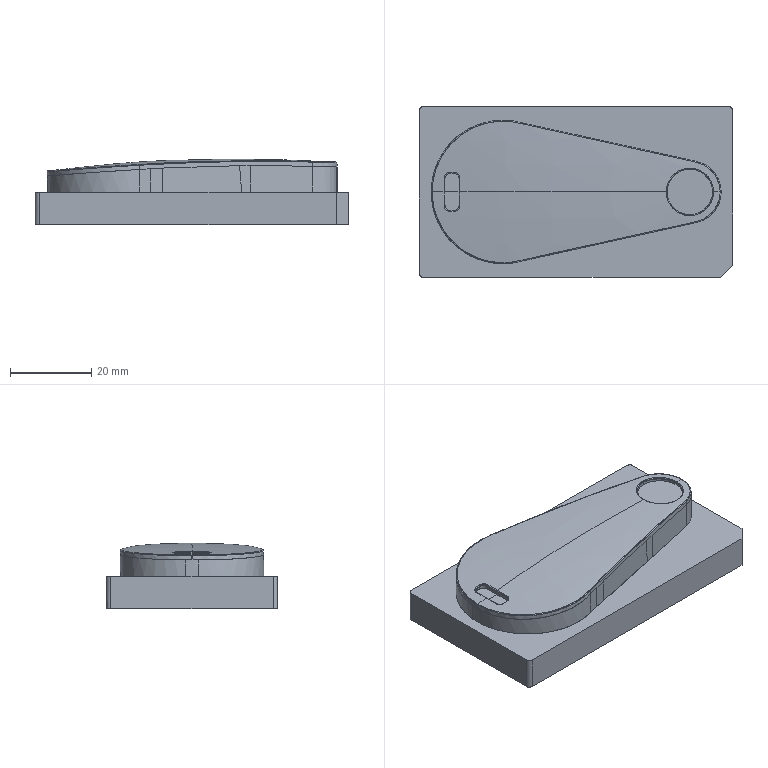NC program | PowerMill | posted with a generic post | part box 77 x 42 x 16.114 mm
Lines 5463 to 6450 of 230441:
N5560 M6
N5561 S18000 M03
N5562 G00 G90 X0.0 Y0.0
N5563 G43 Z9.8037 H2
N5564
N5565 G05 P10000 R4
N5566 X25.6106 Y4.3467
N5567 Z0.8002
N5568 G01 Z-0.3998 F3600.0
N5569 X25.5892 Y4.3418 F6000.0
N5570 G03 X25.4406 Y4.1045 I0.0443 J-0.193
N5571 G01 X25.4866 Y3.9044
N5572 X25.4887 Y3.4164
N5573 X25.3787 Y2.998
N5574 X25.0805 Y2.4403
N5575 X24.5954 Y1.4642
N5576 X24.4343 Y0.9761
N5577 X24.3483 Y0.4881
N5578 X24.3167 Y0.0
N5579 X24.3478 Y-0.4881
N5580 X24.4026 Y-0.8353
N5581 X24.5953 Y-1.4642
N5582 X24.8242 Y-1.9522
N5583 X25.3481 Y-2.9283
N5584 X25.4887 Y-3.4164
N5585 X25.4785 Y-3.9044
N5586 X25.4342 Y-4.1119
N5587 G00 Z3.6074
N5588 G01 X27.1301 Y-2.5287 F10000.0
N5589 G00 Z0.6074
N5590 G01 Z-0.5926 F3600.0
N5591 X27.116 Y-2.5456 F6000.0
N5592 G03 X27.1414 Y-2.8245 I0.1521 J-0.1268
N5593 G01 X28.3826 Y-3.8587
N5594 X28.5768 Y-3.9044
N5595 X28.7951 Y-4.0192
N5596 X29.3579 Y-4.3925
N5597 X29.7167 Y-4.8805
N5598 X29.9105 Y-5.3686
N5599 X29.9759 Y-5.8566
N5600 X29.7712 Y-6.6239
N5601 X29.2812 Y-7.3208
N5602 X28.8585 Y-7.8088
N5603 X28.8118 Y-7.8327
N5604 X28.7708 Y-7.8653
N5605 X28.3555 Y-8.2969
N5606 X27.3258 Y-9.273
N5607 X26.8429 Y-9.654
N5608 X26.3548 Y-9.9782
N5609 X25.8668 Y-10.1481
N5610 X23.9146 Y-10.6849
N5611 X19.5221 Y-11.695
N5612 X12.2013 Y-13.2735
N5613 X9.9964 Y-13.6655
N5614 X9.7611 Y-13.6988
N5615 X9.273 Y-13.7039
N5616 X7.8088 Y-13.6203
N5617 X6.8327 Y-13.5369
N5618 X2.4403 Y-12.8888
N5619 X1.4642 Y-12.6222
N5620 X0.225 Y-12.2013
N5621 X-2.4782 Y-11.2252
N5622 X-4.1922 Y-10.2491
N5623 X-6.6783 Y-8.2969
N5624 X-7.2227 Y-7.8088
N5625 X-7.5763 Y-7.3208
N5626 X-8.8466 Y-5.3686
N5627 X-9.0736 Y-4.8805
N5628 X-9.2569 Y-4.3925
N5629 X-9.273 Y-4.2801
N5630 X-9.4151 Y-3.9044
N5631 X-9.7611 Y-2.7958
N5632 X-9.8455 Y-2.4403
N5633 X-10.12 Y0.0
N5634 X-10.0611 Y0.4881
N5635 X-9.5893 Y3.4164
N5636 X-9.4579 Y3.9044
N5637 X-9.2392 Y4.3925
N5638 X-8.4707 Y5.8566
N5639 X-8.2969 Y6.2312
N5640 X-7.7643 Y7.0243
N5641 X-7.2192 Y7.8088
N5642 X-6.8327 Y8.1753
N5643 X-6.3447 Y8.5793
N5644 X-4.2536 Y10.2491
N5645 X-2.9283 Y11.0116
N5646 X-2.4011 Y11.2252
N5647 X0.9761 Y12.5318
N5648 X1.6269 Y12.6894
N5649 X5.3686 Y13.3735
N5650 X7.8088 Y13.6136
N5651 X9.273 Y13.7182
N5652 X9.7611 Y13.7068
N5653 X12.2013 Y13.2736
N5654 X19.4399 Y11.7133
N5655 X24.4026 Y10.5617
N5656 X25.8668 Y10.1488
N5657 X26.3548 Y9.9675
N5658 X26.6924 Y9.7611
N5659 X27.8709 Y8.7849
N5660 X28.3071 Y8.3429
N5661 X28.3784 Y8.2969
N5662 X28.7951 Y7.8593
N5663 X29.2752 Y7.3208
N5664 X29.7712 Y6.6241
N5665 X29.9436 Y5.8566
N5666 X29.9106 Y5.3686
N5667 X29.7167 Y4.8805
N5668 X29.3579 Y4.3925
N5669 X28.7951 Y4.0127
N5670 X28.5768 Y3.9044
N5671 X27.819 Y3.7276
N5672 X27.331 Y3.636
N5673 X26.8429 Y3.4818
N5674 X26.3548 Y3.2494
N5675 X25.8668 Y2.9362
N5676 X25.3787 Y2.5085
N5677 X24.95 Y1.9522
N5678 X24.6865 Y1.4642
N5679 X24.5104 Y0.9761
N5680 X24.4102 Y0.4881
N5681 X24.3727 Y0.0
N5682 X24.4026 Y-0.4368
N5683 X24.5106 Y-0.9761
N5684 X24.6871 Y-1.4642
N5685 X24.95 Y-1.9522
N5686 X25.3787 Y-2.5062
N5687 X25.8513 Y-2.9283
N5688 X26.3548 Y-3.2502
N5689 X26.6937 Y-3.4164
N5690 X27.331 Y-3.6387
N5691 X27.3463 Y-3.6415
N5692 X27.819 Y-3.7262
N5693 X28.3826 Y-3.8587
N5694 G00 Z3.4146
N5695 G01 X35.8789 Y-0.8619 F10000.0
N5696 G00 Z0.4146
N5697 G01 Z-0.7854 F3600.0
N5698 X35.6662 Y-0.9181 F6000.0
N5699 X35.1553 Y-1.0529
N5700 X35.2638 Y-1.4642
N5701 X35.3532 Y-1.9522
N5702 X35.3635 Y-2.4403
N5703 X35.2988 Y-2.9283
N5704 X35.0735 Y-3.9044
N5705 X34.6517 Y-5.2467
N5706 X33.9876 Y-6.8327
N5707 X33.6756 Y-7.3561
N5708 X33.3034 Y-7.8088
N5709 X32.6995 Y-8.2555
N5710 X32.2115 Y-8.5608
N5711 X31.7554 Y-8.7849
N5712 X30.7473 Y-9.1776
N5713 X29.7712 Y-9.4515
N5714 X26.3135 Y-10.2491
N5715 X16.5938 Y-12.3992
N5716 X5.8566 Y-14.7403
N5717 X4.3934 Y-15.0298
N5718 X2.9283 Y-15.3093
N5719 X1.9522 Y-15.4353
N5720 X1.4642 Y-15.451
N5721 X0.4881 Y-15.2623
N5722 X-1.9522 Y-14.6462
N5723 X-2.4403 Y-14.4911
N5724 X-3.246 Y-14.1535
N5725 X-3.4164 Y-14.0596
N5726 X-4.3925 Y-13.6327
N5727 X-5.4918 Y-13.1774
N5728 X-6.3447 Y-12.7858
N5729 X-6.8327 Y-12.5383
N5730 X-7.8088 Y-11.7777
N5731 X-9.5744 Y-10.2491
N5732 X-10.0631 Y-9.7611
N5733 X-10.7372 Y-8.9567
N5734 X-11.7133 Y-7.574
N5735 X-11.8564 Y-7.3208
N5736 X-12.2728 Y-6.3447
N5737 X-12.8568 Y-4.8805
N5738 X-13.4383 Y-2.4403
N5739 X-13.5139 Y-1.4642
N5740 X-13.6555 Y0.0
N5741 X-13.2625 Y3.4164
N5742 X-13.1774 Y3.8738
N5743 X-13.0029 Y4.3925
N5744 X-12.1989 Y6.3447
N5745 X-11.8442 Y7.3208
N5746 X-11.7133 Y7.556
N5747 X-10.8773 Y8.7849
N5748 X-10.0633 Y9.7611
N5749 X-9.7611 Y10.0829
N5750 X-8.7849 Y11.0004
N5751 X-7.3131 Y12.2013
N5752 X-6.8327 Y12.5382
N5753 X-6.3447 Y12.7951
N5754 X-4.482 Y13.6655
N5755 X-2.9283 Y14.323
N5756 X-0.9761 Y14.8925
N5757 X0.4881 Y15.2705
N5758 X1.4642 Y15.4511
N5759 X1.9522 Y15.4349
N5760 X2.9283 Y15.3086
N5761 X5.8566 Y14.7382
N5762 X7.8088 Y14.3235
N5763 X23.9146 Y10.7827
N5764 X29.7712 Y9.4523
N5765 X30.7473 Y9.1777
N5766 X31.7234 Y8.7999
N5767 X32.2115 Y8.5582
N5768 X32.6995 Y8.2553
N5769 X33.3046 Y7.8088
N5770 X33.6756 Y7.3973
N5771 X33.9847 Y6.8327
N5772 X34.4222 Y5.8566
N5773 X34.6155 Y5.3686
N5774 X34.9322 Y4.3925
N5775 X35.2987 Y2.9283
N5776 X35.3635 Y2.4403
N5777 X35.3532 Y1.9522
N5778 X35.2638 Y1.4642
N5779 X35.1398 Y1.0387
N5780 X35.0622 Y0.9761
N5781 X34.6517 Y0.427
N5782 X34.1637 Y0.1714
N5783 X33.6756 Y0.0491
N5784 X33.1876 Y0.0475
N5785 X32.6995 Y0.1706
N5786 X32.2529 Y0.4881
N5787 X31.7234 Y0.9959
N5788 X31.482 Y1.4642
N5789 X31.2354 Y1.8465
N5790 X30.7585 Y2.4403
N5791 X30.2593 Y2.8756
N5792 X29.7712 Y3.1695
N5793 X29.2832 Y3.3861
N5794 X28.7951 Y3.528
N5795 X28.4637 Y3.5738
N5796 X28.2514 Y1.7284
N5797 G02 X29.5105 Y0.833 I-0.183 J-1.5903
N5798 G01 X29.7351 Y0.367
N5799 G02 X29.7651 Y-0.2566 I-0.7207 J-0.3473
N5800 G01 X29.617 Y-0.6592
N5801 G02 X26.5398 Y-0.3983 I-1.5028 J0.5532
N5802 G01 X26.4945 Y-0.1541
N5803 G02 X28.2514 Y1.7284 I1.5739 J0.2922
N5804 G01 X28.4637 Y3.5738
N5805 X28.3071 Y3.5954
N5806 X27.819 Y3.5943
N5807 X27.331 Y3.5453
N5808 X26.8429 Y3.421
N5809 X26.3548 Y3.2163
N5810 X25.8819 Y2.9283
N5811 X25.3787 Y2.4945
N5812 X24.95 Y1.9522
N5813 X24.6868 Y1.4642
N5814 X24.5104 Y0.9761
N5815 X24.4102 Y0.4881
N5816 X24.3727 Y0.0
N5817 X24.4026 Y-0.4366
N5818 X24.5143 Y-0.9761
N5819 X24.6822 Y-1.4503
N5820 X24.6878 Y-1.4644
N5821 X24.6945 Y-1.478
N5822 X24.9109 Y-1.8796
N5823 X25.3787 Y-2.4942
N5824 X25.8668 Y-2.9171
N5825 X26.3548 Y-3.2156
N5826 X26.838 Y-3.4164
N5827 X27.331 Y-3.5441
N5828 X27.819 Y-3.5974
N5829 X28.3071 Y-3.5959
N5830 X28.7951 Y-3.528
N5831 X29.2013 Y-3.4164
N5832 X29.7712 Y-3.1695
N5833 X30.1837 Y-2.9283
N5834 X30.513 Y-2.6751
N5835 X30.7473 Y-2.451
N5836 X31.1615 Y-1.9522
N5837 X31.482 Y-1.4642
N5838 X31.7295 Y-0.9761
N5839 X32.2115 Y-0.4065
N5840 X32.6995 Y-0.1452
N5841 X33.1876 Y-0.0416
N5842 X33.6756 Y-0.044
N5843 X34.1637 Y-0.1484
N5844 X34.6817 Y-0.4881
N5845 X35.0187 Y-0.9203
N5846 X35.0641 Y-0.9629
N5847 X35.1208 Y-0.9884
N5848 X35.1302 Y-0.9915
N5849 X35.1398 Y-0.9941
N5850 X35.1553 Y-1.0529
N5851 X35.6662 Y-0.9181
N5852 X38.5413 Y0.1203 Z-0.9782
N5853 X38.5227 Y0.1321
N5854 G03 X38.2495 Y0.0705 I-0.1058 J-0.1674
N5855 G01 X37.508 Y-1.1028
N5856 X37.4718 Y-1.4642
N5857 X37.2745 Y-2.4403
N5858 X36.9717 Y-3.4164
N5859 X36.604 Y-4.2751
N5860 X36.1159 Y-5.1424
N5861 X35.6243 Y-5.8566
N5862 X35.2324 Y-6.3447
N5863 X34.7776 Y-6.8327
N5864 X34.2506 Y-7.3208
N5865 X33.6405 Y-7.8088
N5866 X32.9051 Y-8.2969
N5867 X31.9708 Y-8.7849
N5868 X31.2354 Y-9.0837
N5869 X30.2593 Y-9.3761
N5870 X26.4891 Y-10.2085
N5871 X26.4882 Y-10.2088
N5872 X26.3135 Y-10.2491
N5873 X16.5938 Y-12.3992
N5874 X14.5691 Y-12.8406
N5875 X1.9925 Y-15.6177
N5876 X-0.4881 Y-16.1386
N5877 X-2.4403 Y-16.5026
N5878 X-3.2654 Y-16.5938
N5879 X-3.9044 Y-16.5999
N5880 X-4.3925 Y-16.4683
N5881 X-6.3447 Y-15.7841
N5882 X-6.7264 Y-15.6177
N5883 X-8.7849 Y-14.5464
N5884 X-10.7372 Y-13.2261
N5885 X-11.7133 Y-12.294
N5886 X-11.837 Y-12.2013
N5887 X-12.2013 Y-11.7945
N5888 X-13.6655 Y-9.9471
N5889 X-14.1139 Y-9.273
N5890 X-14.6628 Y-8.2969
N5891 X-15.1116 Y-7.3208
N5892 X-15.5806 Y-5.8566
N5893 X-15.8781 Y-4.8805
N5894 X-15.9874 Y-4.3925
N5895 X-16.3348 Y-2.4403
N5896 X-16.4619 Y-0.4881
N5897 X-16.5158 Y0.0
N5898 X-16.2262 Y3.4164
N5899 X-15.9983 Y4.3925
N5900 X-15.4109 Y6.3447
N5901 X-15.296 Y6.8327
N5902 X-15.1247 Y7.3208
N5903 X-14.4132 Y8.7849
N5904 X-14.1374 Y9.273
N5905 X-13.8175 Y9.7611
N5906 X-13.0974 Y10.7372
N5907 X-12.285 Y11.7133
N5908 X-11.8245 Y12.208
N5909 X-11.3501 Y12.6894
N5910 X-10.7372 Y13.2181
N5911 X-9.4035 Y14.1535
N5912 X-8.7849 Y14.5248
N5913 X-6.8327 Y15.5703
N5914 X-6.3447 Y15.7858
N5915 X-4.3925 Y16.4679
N5916 X-3.9044 Y16.5929
N5917 X-3.4164 Y16.6082
N5918 X-2.4403 Y16.5026
N5919 X-0.4881 Y16.1392
N5920 X1.4642 Y15.7293
N5921 X29.2832 Y9.6002
N5922 X30.6571 Y9.273
N5923 X31.2354 Y9.0811
N5924 X31.9708 Y8.7849
N5925 X32.9053 Y8.2969
N5926 X33.6756 Y7.7844
N5927 X34.2507 Y7.3208
N5928 X34.6517 Y6.9583
N5929 X35.1398 Y6.4481
N5930 X35.6278 Y5.8512
N5931 X35.9751 Y5.3686
N5932 X36.5433 Y4.3925
N5933 X36.7728 Y3.9044
N5934 X37.092 Y3.0703
N5935 X37.2745 Y2.4403
N5936 X37.4718 Y1.4642
N5937 X37.5697 Y0.4881
N5938 Y-0.4881
N5939 X37.508 Y-1.1028
N5940 X38.6013 Y0.1297 Z-1.171
N5941 X38.5827 Y0.1415
N5942 G03 X38.3094 Y0.0807 I-0.1063 J-0.1671
N5943 G01 X37.5534 Y-1.1075
N5944 X37.5165 Y-1.4642
N5945 X37.3193 Y-2.4403
N5946 X37.092 Y-3.1878
N5947 X36.8083 Y-3.9044
N5948 X36.604 Y-4.3287
N5949 X36.1159 Y-5.1943
N5950 X35.6525 Y-5.8566
N5951 X35.2503 Y-6.3447
N5952 X34.796 Y-6.8327
N5953 X34.274 Y-7.3208
N5954 X33.6756 Y-7.7972
N5955 X33.1876 Y-8.1303
N5956 X32.9821 Y-8.2457
N5957 X32.9051 Y-8.2969
N5958 X32.7049 Y-8.4014
N5959 X32.2115 Y-8.6785
N5960 X31.7234 Y-8.9028
N5961 X31.3486 Y-9.0377
N5962 X31.25 Y-9.0785
N5963 X31.1479 Y-9.1099
N5964 X30.7473 Y-9.254
N5965 X30.2593 Y-9.3836
N5966 X2.0338 Y-15.6177
N5967 X-4.7201 Y-17.0818
N5968 X-6.8327 Y-17.4646
N5969 X-7.8088 Y-17.5274
N5970 X-8.2969 Y-17.4459
N5971 X-9.273 Y-17.0261
N5972 X-10.178 Y-16.5938
N5973 X-11.2252 Y-15.9695
N5974 X-13.0937 Y-14.6416
N5975 X-13.6831 Y-14.1535
N5976 X-14.1434 Y-13.6655
N5977 X-14.6416 Y-13.085
N5978 X-15.6177 Y-11.8131
N5979 X-15.9656 Y-11.2252
N5980 X-17.0688 Y-9.273
N5981 X-17.87 Y-7.3208
N5982 X-18.0273 Y-6.8327
N5983 X-18.0579 Y-6.6332
N5984 X-18.3548 Y-5.3686
N5985 X-18.5641 Y-4.3925
N5986 X-18.8405 Y-2.4403
N5987 X-18.9401 Y-0.4881
N5988 X-18.9947 Y0.0
N5989 X-18.7456 Y3.4164
N5990 X-18.6554 Y3.9044
N5991 X-18.1008 Y6.3447
N5992 X-18.0279 Y6.8327
N5993 X-17.8698 Y7.3208
N5994 X-17.3047 Y8.7849
N5995 X-17.0692 Y9.273
N5996 X-16.3013 Y10.7372
N5997 X-15.6904 Y11.7133
N5998 X-15.3542 Y12.2013
N5999 X-14.972 Y12.6894
N6000 X-14.1378 Y13.6655
N6001 X-13.617 Y14.1535
N6002 X-12.4526 Y15.1296
N6003 X-11.0551 Y16.1057
N6004 X-10.2491 Y16.5623
N6005 X-9.273 Y17.0172
N6006 X-8.2969 Y17.4437
N6007 X-7.8088 Y17.5226
N6008 X-6.8327 Y17.4637
N6009 X-5.3686 Y17.2116
N6010 X-2.9283 Y16.7055
N6011 X29.7712 Y9.4991
N6012 X30.7473 Y9.2539
N6013 X31.1362 Y9.114
N6014 X31.2354 Y9.0811
N6015 X31.2998 Y9.0551
N6016 X31.3033 Y9.0539
N6017 X31.7234 Y8.9027
N6018 X32.2115 Y8.6784
N6019 X32.916 Y8.2969
N6020 X33.6597 Y7.8088
N6021 X34.1637 Y7.4134
N6022 X34.6517 Y6.9725
N6023 X35.1398 Y6.4705
N6024 X35.6278 Y5.8863
N6025 X36.0046 Y5.3686
N6026 X36.3045 Y4.8805
N6027 X36.8083 Y3.9044
N6028 X37.004 Y3.4164
N6029 X37.3193 Y2.4403
N6030 X37.429 Y1.9522
N6031 X37.5815 Y0.9761
N6032 X37.6135 Y0.4881
N6033 X37.6174 Y-0.4881
N6034 X37.5534 Y-1.1075
N6035 X38.6068 Y0.1353 Z-1.3639
N6036 X38.5882 Y0.147
N6037 G03 X38.3151 Y0.0853 I-0.1057 J-0.1674
N6038 G01 X37.5614 Y-1.1083
N6039 X37.5259 Y-1.4642
N6040 X37.3269 Y-2.4403
N6041 X37.1808 Y-2.9283
N6042 X37.0014 Y-3.4176
N6043 X36.8156 Y-3.9044
N6044 X36.6977 Y-4.1339
N6045 X36.6209 Y-4.296
N6046 X36.5338 Y-4.4529
N6047 X36.3142 Y-4.8805
N6048 X36.0126 Y-5.3686
N6049 X35.6278 Y-5.898
N6050 X35.2593 Y-6.3447
N6051 X34.8056 Y-6.8327
N6052 X34.2845 Y-7.3208
N6053 X33.6756 Y-7.806
N6054 X33.1876 Y-8.1387
N6055 X32.2115 Y-8.686
N6056 X31.7234 Y-8.9104
N6057 X30.7473 Y-9.2609
N6058 X30.2646 Y-9.3821
N6059 X30.2593 Y-9.3835
N6060 X30.2567 Y-9.3841
N6061 X29.7712 Y-9.506
N6062 X5.213 Y-14.9155
N6063 X2.0338 Y-15.6176
N6064 X1.4894 Y-15.7357
N6065 X-6.8378 Y-17.5699
N6066 X-9.2306 Y-18.0579
N6067 X-10.2491 Y-18.2271
N6068 X-11.2252 Y-18.2888
N6069 X-11.7133 Y-18.2104
N6070 X-12.0948 Y-18.0579
N6071 X-13.1774 Y-17.4667
N6072 X-15.1296 Y-16.0148
N6073 X-15.5847 Y-15.6177
N6074 X-16.1057 Y-15.1097
N6075 X-16.5938 Y-14.5842
N6076 X-17.0818 Y-14.0032
N6077 X-17.6707 Y-13.1774
N6078 X-18.546 Y-11.6747
N6079 X-18.7707 Y-11.2252
N6080 X-19.6163 Y-9.273
N6081 X-20.0737 Y-7.8088
N6082 X-20.3998 Y-6.8327
N6083 X-20.8489 Y-4.3925
N6084 X-21.0714 Y-2.4403
N6085 X-21.1949 Y0.0
N6086 X-20.9872 Y3.4164
N6087 X-20.6577 Y5.3686
N6088 X-20.5507 Y5.8566
N6089 X-20.3912 Y6.8327
N6090 X-19.9648 Y8.2969
N6091 X-19.6171 Y9.273
N6092 X-19.2321 Y10.2491
N6093 X-18.5389 Y11.7133
N6094 X-17.671 Y13.1774
N6095 X-17.3329 Y13.6655
N6096 X-16.9286 Y14.1535
N6097 X-16.0646 Y15.1296
N6098 X-15.1296 Y16.0113
N6099 X-14.1535 Y16.8025
N6100 X-13.7364 Y17.0818
N6101 X-12.1179 Y18.0579
N6102 X-11.7133 Y18.2193
N6103 X-11.2252 Y18.2857
N6104 X-10.2491 Y18.2268
N6105 X-9.2306 Y18.0579
N6106 X-7.3208 Y17.6744
N6107 X29.7712 Y9.506
N6108 X30.7473 Y9.2611
N6109 X31.7234 Y8.9101
N6110 X32.2115 Y8.6859
N6111 X32.9296 Y8.2969
N6112 X33.671 Y7.8088
N6113 X34.2835 Y7.3208
N6114 X34.6517 Y6.9811
N6115 X35.1398 Y6.4808
N6116 X35.6278 Y5.8978
N6117 X36.0126 Y5.3686
N6118 X36.3124 Y4.8805
N6119 X36.8156 Y3.9044
N6120 X37.092 Y3.2071
N6121 X37.3269 Y2.4403
N6122 X37.4013 Y2.075
N6123 X37.429 Y1.9522
N6124 X37.4374 Y1.8981
N6125 X37.4383 Y1.8936
N6126 X37.5259 Y1.4642
N6127 X37.585 Y0.9761
N6128 X37.6061 Y0.6008
N6129 X37.6135 Y0.4881
N6130 X37.6136 Y0.4674
N6131 X37.6397 Y0.0
N6132 X37.6234 Y-0.4881
N6133 X37.5614 Y-1.1083
N6134 X38.6137 Y0.1393 Z-1.5567
N6135 X38.5951 Y0.151
N6136 G03 X38.3221 Y0.089 I-0.1055 J-0.1675
N6137 G01 X37.5679 Y-1.1089
N6138 X37.5329 Y-1.4642
N6139 X37.3338 Y-2.4403
N6140 X37.092 Y-3.2278
N6141 X36.8229 Y-3.9044
N6142 X36.322 Y-4.8805
N6143 X36.0206 Y-5.3686
N6144 X35.6278 Y-5.9095
N6145 X35.268 Y-6.3447
N6146 X34.8152 Y-6.8327
N6147 X34.295 Y-7.3208
N6148 X33.6835 Y-7.8088
N6149 X33.1876 Y-8.1469
N6150 X32.2115 Y-8.6934
N6151 X31.7234 Y-8.9179
N6152 X30.7473 Y-9.2679
N6153 X30.2593 Y-9.3978
N6154 X18.546 Y-11.9966
N6155 X-1.0539 Y-16.2958
N6156 X-6.8378 Y-17.5698
N6157 X-7.1853 Y-17.6407
N6158 X-7.1867 Y-17.641
N6159 X-11.3124 Y-18.546
N6160 X-13.1774 Y-18.9116
N6161 X-13.6655 Y-18.9711
N6162 X-14.1535 Y-18.9771
N6163 X-14.6416 Y-18.9009
N6164 X-15.1296 Y-18.7063
N6165 X-16.1057 Y-18.0512
N6166 X-16.5993 Y-17.6588
N6167 X-17.0818 Y-17.2529
N6168 X-18.7028 Y-15.6177
N6169 X-19.0773 Y-15.1296
N6170 X-20.0511 Y-13.6655
N6171 X-20.806 Y-12.2013
N6172 X-21.2281 Y-11.2252
N6173 X-21.8994 Y-9.273
N6174 X-22.407 Y-7.3208
N6175 X-22.5563 Y-6.8327
N6176 X-22.9499 Y-4.3925
N6177 X-23.1352 Y-2.4403
N6178 X-23.2321 Y0.0
N6179 X-23.053 Y3.4164
N6180 X-22.5459 Y6.8327
N6181 X-22.3146 Y7.8088
N6182 X-21.9002 Y9.273
N6183 X-21.4024 Y10.7372
N6184 X-21.0306 Y11.7133
N6185 X-20.3121 Y13.1774
N6186 X-19.4051 Y14.6416
N6187 X-18.6695 Y15.6177
N6188 X-18.2614 Y16.1057
N6189 X-17.31 Y17.0818
N6190 X-16.7165 Y17.5699
N6191 X-15.1296 Y18.7067
N6192 X-14.6416 Y18.9097
N6193 X-14.1535 Y18.9796
N6194 X-13.6655 Y18.9706
N6195 X-13.1774 Y18.9121
N6196 X-10.2491 Y18.3212
N6197 X29.7712 Y9.5129
N6198 X30.7473 Y9.2684
N6199 X31.7234 Y8.9175
N6200 X32.2115 Y8.6933
N6201 X32.9433 Y8.2969
N6202 X33.6756 Y7.8136
N6203 X34.2943 Y7.3208
N6204 X34.6517 Y6.9905
N6205 X35.1398 Y6.491
N6206 X35.6278 Y5.9093
N6207 X36.0206 Y5.3686
N6208 X36.3203 Y4.8805
N6209 X36.8229 Y3.9044
N6210 X37.092 Y3.2274
N6211 X37.3338 Y2.4403
N6212 X37.5329 Y1.4642
N6213 X37.591 Y0.9761
N6214 X37.6465 Y0.0
N6215 X37.6291 Y-0.4881
N6216 X37.5679 Y-1.1089
N6217 X38.622 Y0.0366 Z-1.7532
N6218 X38.6037 Y0.0489
N6219 G03 X38.3289 Y-0.005 I-0.1104 J-0.1644
N6220 G01 X37.5856 Y-1.1112
N6221 X37.5401 Y-1.4642
N6222 X37.3409 Y-2.4403
N6223 X37.092 Y-3.2477
N6224 X36.8303 Y-3.9044
N6225 X36.33 Y-4.8805
N6226 X36.0288 Y-5.3686
N6227 X35.6278 Y-5.9211
N6228 X35.277 Y-6.3447
N6229 X34.825 Y-6.8327
N6230 X34.3057 Y-7.3208
N6231 X33.6952 Y-7.8088
N6232 X33.1876 Y-8.1552
N6233 X32.6995 Y-8.4428
N6234 X32.3511 Y-8.6152
N6235 X32.2115 Y-8.6934
N6236 X31.9658 Y-8.8061
N6237 X31.7234 Y-8.9257
N6238 X30.7473 Y-9.2749
N6239 X30.2814 Y-9.3919
N6240 X30.2593 Y-9.3978
N6241 X30.2477 Y-9.4003
N6242 X29.7712 Y-9.5199
N6243 X22.0982 Y-11.2085
N6244 X18.546 Y-11.9966
N6245 X9.5792 Y-13.9634
N6246 X-12.2013 Y-18.7565
N6247 X-13.2866 Y-19.0341
N6248 X-14.6416 Y-19.2976
N6249 X-15.6177 Y-19.4108
N6250 X-16.5938 Y-19.4465
N6251 X-17.0818 Y-19.4033
N6252 X-17.5699 Y-19.3145
N6253 X-18.0579 Y-19.1191
N6254 X-18.546 Y-18.7445
N6255 X-19.5221 Y-17.8669
N6256 X-20.2657 Y-17.0818
N6257 X-21.4743 Y-15.4946
N6258 X-21.7219 Y-15.1296
N6259 X-22.7094 Y-13.1774
N6260 X-23.4812 Y-11.2252
N6261 X-23.6449 Y-10.7372
N6262 X-24.1842 Y-8.7849
N6263 X-24.6862 Y-6.3447
N6264 X-24.9597 Y-4.3925
N6265 X-25.1206 Y-2.4403
N6266 X-25.1937 Y0.0
N6267 X-25.0396 Y3.4164
N6268 X-24.6767 Y6.3447
N6269 X-24.5036 Y7.3208
N6270 X-24.1852 Y8.7849
N6271 X-23.6451 Y10.7372
N6272 X-23.4819 Y11.2252
N6273 X-22.9152 Y12.6894
N6274 X-22.229 Y14.1535
N6275 X-21.3856 Y15.6177
N6276 X-20.6908 Y16.5938
N6277 X-20.2979 Y17.0818
N6278 X-19.0341 Y18.2641
N6279 X-18.1893 Y19.0341
N6280 X-18.0579 Y19.1181
N6281 X-17.5699 Y19.3183
N6282 X-17.0818 Y19.4017
N6283 X-16.5938 Y19.4451
N6284 X-16.1057 Y19.4348
N6285 X-15.1296 Y19.3676
N6286 X-13.6655 Y19.1217
N6287 X-12.6894 Y18.875
N6288 X-12.6864 Y18.8744
N6289 X29.7712 Y9.5199
N6290 X30.7536 Y9.273
N6291 X31.7234 Y8.9251
N6292 X32.2115 Y8.7009
N6293 X32.9572 Y8.2969
N6294 X33.6947 Y7.8088
N6295 X34.3052 Y7.3208
N6296 X34.6517 Y7.0
N6297 X35.1398 Y6.5014
N6298 X35.6278 Y5.921
N6299 X36.0288 Y5.3686
N6300 X36.3283 Y4.8805
N6301 X36.8303 Y3.9044
N6302 X37.092 Y3.2482
N6303 X37.3409 Y2.4403
N6304 X37.5401 Y1.4642
N6305 X37.5989 Y0.9761
N6306 X37.6533 Y0.0
N6307 X37.6311 Y-0.4314
N6308 X37.6291 Y-0.488
N6309 X37.6272 Y-0.5074
N6310 X37.603 Y-0.9761
N6311 X37.5856 Y-1.1112
N6312 X38.6289 Y0.0352 Z-1.9498
N6313 X38.6106 Y0.0475
N6314 G03 X38.3358 Y-0.0064 I-0.1104 J-0.1643
N6315 G01 X37.5927 Y-1.1121
N6316 X37.5473 Y-1.4642
N6317 X37.348 Y-2.4403
N6318 X37.092 Y-3.2675
N6319 X36.8377 Y-3.9044
N6320 X36.3379 Y-4.8805
N6321 X36.0369 Y-5.3686
N6322 X35.6278 Y-5.9328
N6323 X35.2859 Y-6.3447
N6324 X34.8347 Y-6.8327
N6325 X34.3164 Y-7.3208
N6326 X33.707 Y-7.8088
N6327 X33.1876 Y-8.1602
N6328 X32.6995 Y-8.4507
N6329 X32.2309 Y-8.6824
N6330 X32.2114 Y-8.6933
N6331 X32.1745 Y-8.7103
N6332 X31.7234 Y-8.9334
N6333 X30.7838 Y-9.273
N6334 X30.1907 Y-9.427
N6335 X29.5924 Y-9.5592
N6336 X3.4164 Y-15.342
N6337 X-12.2013 Y-18.764
N6338 X-13.1774 Y-19.0102
N6339 X-13.2684 Y-19.0293
N6340 X-13.2866 Y-19.034
N6341 X-13.3385 Y-19.0441
N6342 X-14.6416 Y-19.3183
N6343 X-16.2652 Y-19.5221
N6344 X-17.0818 Y-19.5745
N6345 X-18.0579 Y-19.5775
N6346 X-19.0115 Y-19.5221
N6347 X-20.0102 Y-19.3812
N6348 X-20.4982 Y-19.2518
N6349 X-20.9863 Y-19.0717
N6350 X-21.4743 Y-18.7351
N6351 X-21.6585 Y-18.546
N6352 X-22.4504 Y-17.6305
N6353 X-23.1894 Y-16.5938
N6354 X-23.9146 Y-15.3777
N6355 X-24.298 Y-14.6416
N6356 X-24.9014 Y-13.1774
N6357 X-25.2145 Y-12.1976
N6358 X-25.55 Y-11.2252
N6359 X-25.6951 Y-10.7372
N6360 X-26.1937 Y-8.7849
N6361 X-26.5584 Y-6.8327
N6362 X-26.8855 Y-4.3925
N6363 X-27.031 Y-2.4403
N6364 X-27.1037 Y0.0
N6365 X-26.9691 Y3.4164
N6366 X-26.6341 Y6.3447
N6367 X-26.192 Y8.7849
N6368 X-25.6957 Y10.7372
N6369 X-25.2427 Y12.2013
N6370 X-24.8892 Y13.1774
N6371 X-24.4026 Y14.3564
N6372 X-24.0433 Y15.1296
N6373 X-23.5114 Y16.1057
N6374 X-23.2046 Y16.5938
N6375 X-22.8589 Y17.0818
N6376 X-22.0886 Y18.0579
N6377 X-21.4743 Y18.7361
N6378 X-21.0563 Y19.0341
N6379 X-20.4982 Y19.2535
N6380 X-20.0102 Y19.3838
N6381 X-19.0341 Y19.5197
N6382 X-18.0579 Y19.5765
N6383 X-17.0818 Y19.5749
N6384 X-16.5938 Y19.5484
N6385 X-15.1296 Y19.3916
N6386 X-13.6655 Y19.1246
N6387 X-12.6894 Y18.88
N6388 X-12.6866 Y18.8794
N6389 X29.7712 Y9.5256
N6390 X30.7473 Y9.2841
N6391 X31.7234 Y8.9319
N6392 X32.2115 Y8.7084
N6393 X32.9711 Y8.2969
N6394 X33.7069 Y7.8088
N6395 X34.1637 Y7.4459
N6396 X34.2915 Y7.3317
N6397 X34.3051 Y7.3208
N6398 X34.3464 Y7.2826
N6399 X34.6517 Y7.0095
N6400 X35.1398 Y6.5118
N6401 X35.6278 Y5.9327
N6402 X36.0369 Y5.3686
N6403 X36.3364 Y4.8805
N6404 X36.8377 Y3.9044
N6405 X37.092 Y3.2681
N6406 X37.348 Y2.4403
N6407 X37.4581 Y1.9522
N6408 X37.5101 Y1.6107
N6409 X37.5619 Y1.2939
N6410 X37.6069 Y0.9761
N6411 X37.6602 Y0.0
N6412 X37.6102 Y-0.9761
N6413 X37.5927 Y-1.1121
N6414 X38.6328 Y0.0447 Z-2.1464
N6415 X38.6145 Y0.057
N6416 G03 X38.3398 Y0.0029 I-0.1103 J-0.1645
N6417 G01 X37.5917 Y-1.112
N6418 X37.5709 Y-1.2879
N6419 X37.5536 Y-1.4642
N6420 X37.3538 Y-2.4403
N6421 X37.092 Y-3.283
N6422 X36.844 Y-3.9044
N6423 X36.604 Y-4.4071
N6424 X36.3871 Y-4.7844
N6425 X36.1954 Y-5.1232
N6426 X35.9798 Y-5.4473
N6427 X35.6278 Y-5.9414
N6428 X35.2401 Y-6.3907
N6429 X34.8442 Y-6.8327
N6430 X34.3213 Y-7.3208
N6431 X33.711 Y-7.8088
N6432 X33.6271 Y-7.8628
N6433 X33.1876 Y-8.1602
N6434 X32.9409 Y-8.3057
N6435 X32.6995 Y-8.4598
N6436 X31.7234 Y-8.9339
N6437 X30.7838 Y-9.273
N6438 X30.2789 Y-9.4049
N6439 X29.7712 Y-9.5256
N6440 X20.5934 Y-11.5472
N6441 X3.4164 Y-15.3419
N6442 X-6.1071 Y-17.4287
N6443 X-12.2013 Y-18.7711
N6444 X-13.6655 Y-19.1347
N6445 X-14.4294 Y-19.2736
N6446 X-14.5909 Y-19.3097
N6447 X-14.7548 Y-19.3328
N6448 X-15.1296 Y-19.4009
N6449 X-16.2151 Y-19.5221
N6450 X-16.5839 Y-19.5425
N6451 X-17.0818 Y-19.5745
N6452 X-17.1662 Y-19.5748
N6453 X-17.5699 Y-19.5971
N6454 X-19.0341 Y-19.5663
N6455 X-20.0102 Y-19.4812
N6456 X-21.4743 Y-19.2584
N6457 X-22.4504 Y-19.0242
N6458 X-23.4265 Y-18.7027
N6459 X-23.9146 Y-18.462
N6460 X-24.4943 Y-18.0579
N6461 X-24.8907 Y-17.5326
N6462 X-25.4528 Y-16.5938
N6463 X-26.4177 Y-14.6416
N6464 X-26.9456 Y-13.1774
N6465 X-27.6661 Y-10.7372
N6466 X-28.1137 Y-8.7849
N6467 X-28.5324 Y-6.3447
N6468 X-28.7704 Y-4.3925
N6469 X-28.912 Y-2.4403
N6470 X-28.9859 Y0.0
N6471 X-28.9376 Y1.9522
N6472 X-28.8551 Y3.4164
N6473 X-28.5293 Y6.3447
N6474 X-28.1137 Y8.7849
N6475 X-27.6665 Y10.7372
N6476 X-26.9475 Y13.1774
N6477 X-26.4188 Y14.6416
N6478 X-26.2001 Y15.1296
N6479 X-25.453 Y16.5938
N6480 X-24.8635 Y17.5699
N6481 X-24.4026 Y18.1401
N6482 X-23.9146 Y18.4615
N6483 X-23.4265 Y18.6991
N6484 X-22.4504 Y19.0229
N6485 X-21.4743 Y19.2596
N6486 X-20.4982 Y19.4276
N6487 X-19.0341 Y19.5659
N6488 X-18.0579 Y19.5978
N6489 X-17.3326 Y19.5753
N6490 X-16.963 Y19.569
N6491 X-16.5938 Y19.5524
N6492 X-15.1296 Y19.3979
N6493 X-13.6655 Y19.1317
N6494 X-12.6894 Y18.885
N6495 X29.7712 Y9.5256
N6496 X30.7473 Y9.2841
N6497 X31.2354 Y9.1205
N6498 X31.4771 Y9.0203
N6499 X31.7234 Y8.9319
N6500 X31.9656 Y8.8186
N6501 X32.2115 Y8.7138
N6502 X32.9772 Y8.2969
N6503 X33.711 Y7.8088
N6504 X34.1637 Y7.4507
N6505 X34.5061 Y7.1396
N6506 X34.6517 Y7.0095
N6507 X34.67 Y6.9908
N6508 X34.844 Y6.8327
N6509 X35.24 Y6.3906
N6510 X35.6278 Y5.9413
N6511 X36.0421 Y5.3686
N6512 X36.33 Y4.8825
N6513 X36.6111 Y4.3925
N6514 X36.8434 Y3.9044
N6515 X37.092 Y3.2824
N6516 X37.3538 Y2.4403
N6517 X37.4108 Y2.1616
N6518 X37.4461 Y2.0155
N6519 X37.471 Y1.8672
N6520 X37.5533 Y1.4642
N6521 X37.5959 Y1.048
N6522 X37.607 Y0.9744
N6523 X37.611 Y0.9002
N6524 X37.6531 Y0.4881
N6525 X37.6529 Y0.132
N6526 X37.6602 Y-0.0056
N6527 X37.6528 Y-0.1432
N6528 X37.6527 Y-0.4881
N6529 X37.6173 Y-0.8361
N6530 X37.6102 Y-0.9761
N6531 X37.6007 Y-1.044
N6532 X37.5917 Y-1.112
N6533 X38.6328 Y0.0451 Z-2.3429
N6534 X38.6145 Y0.0573
N6535 G03 X38.3398 Y0.0032 I-0.1103 J-0.1644
N6536 G01 X37.5917 Y-1.112
N6537 X37.5709 Y-1.2879
N6538 X37.5536 Y-1.4642
N6539 X37.3538 Y-2.4403
N6540 X37.092 Y-3.2832
N6541 X36.8441 Y-3.9044
N6542 X36.611 Y-4.3925
N6543 X36.6101 Y-4.394
N6544 X36.6039 Y-4.4071
N6545 X36.387 Y-4.7844
N6546 X36.3229 Y-4.907
N6547 X36.2493 Y-5.024